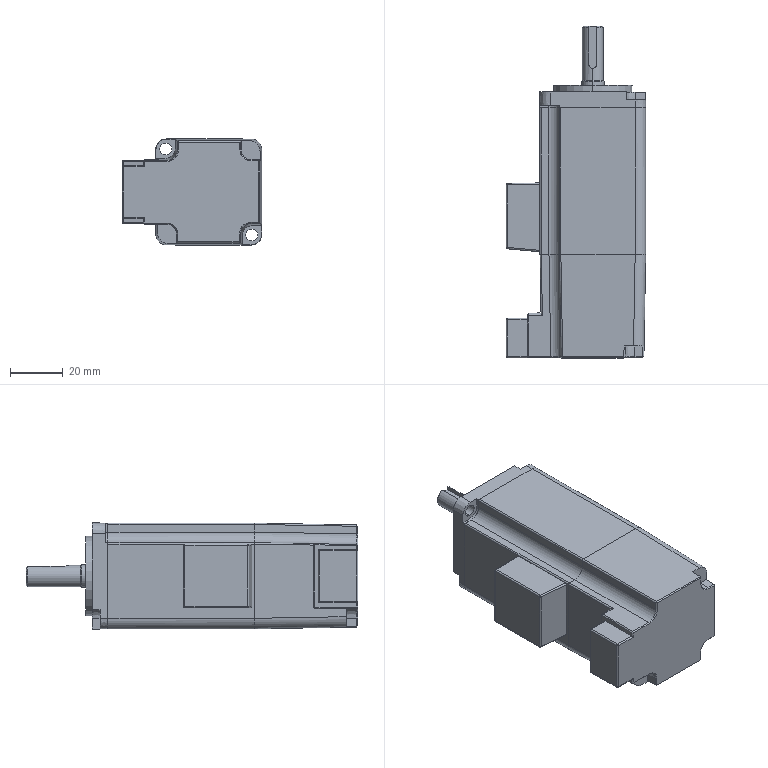Part | STEP file | ECMA_C20401ES | 1 solid | 171 faces | box 52.955 x 125.6 x 40.209 mm | volume 162089 mm3 | plane 88 | cylinder 49 | cone 19 | sphere 8 | spline 7 | commonest cylinder face diameters 1 x24 8 x10 4.5 x4 2 x2 8.5 x2 9 x2